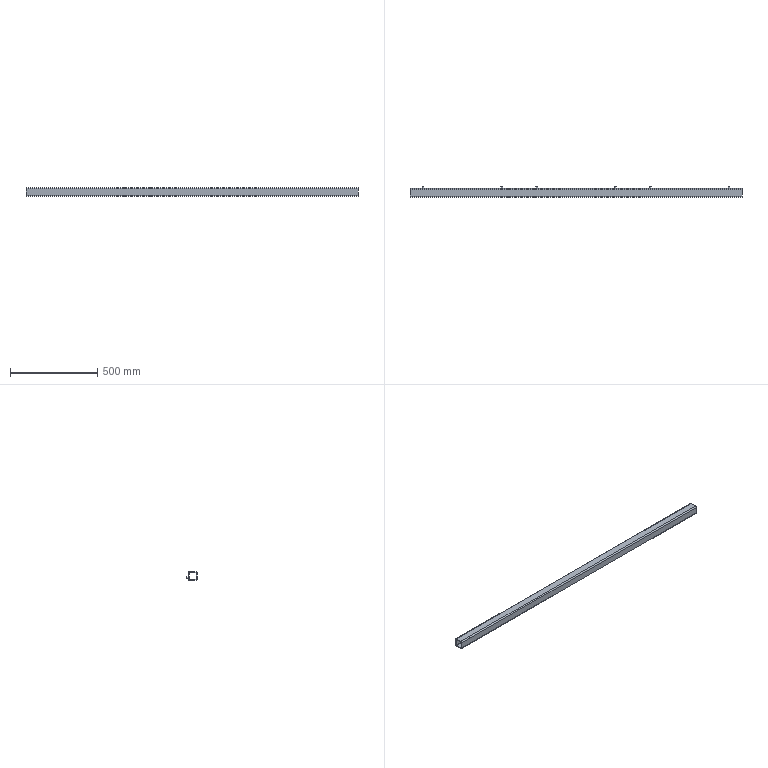Part | NX | 1 solid | 30 faces | box 1900 x 60 x 50 mm | volume 1641319 mm3 | plane 16 | cylinder 14 | commonest cylinder face diameters 10 x6 4 x4 14 x4
STEP:
#1=CARTESIAN_POINT('',(-425.,25.,-590.));
#2=VERTEX_POINT('',#1);
#3=CARTESIAN_POINT('',(-425.,25.,-585.));
#4=DIRECTION('',(0.,-1.,0.));
#5=DIRECTION('',(0.,0.,-1.));
#6=AXIS2_PLACEMENT_3D('',#3,#4,#5);
#7=CIRCLE('',#6,5.);
#8=EDGE_CURVE('',#2,#2,#7,.F.);
#9=ORIENTED_EDGE('',*,*,#8,.F.);
#10=EDGE_LOOP('',(#9));
#11=FACE_BOUND('',#10,.T.);
#12=CARTESIAN_POINT('',(225.,25.,-590.));
#13=VERTEX_POINT('',#12);
#14=CARTESIAN_POINT('',(225.,25.,-585.));
#15=DIRECTION('',(0.,-1.,0.));
#16=DIRECTION('',(0.,0.,-1.));
#17=AXIS2_PLACEMENT_3D('',#14,#15,#16);
#18=CIRCLE('',#17,5.);
#19=EDGE_CURVE('',#13,#13,#18,.F.);
#20=ORIENTED_EDGE('',*,*,#19,.F.);
#21=EDGE_LOOP('',(#20));
#22=FACE_BOUND('',#21,.T.);
#23=CARTESIAN_POINT('',(875.,25.,-590.));
#24=VERTEX_POINT('',#23);
#25=CARTESIAN_POINT('',(875.,25.,-585.));
#26=DIRECTION('',(0.,-1.,0.));
#27=DIRECTION('',(0.,0.,-1.));
#28=AXIS2_PLACEMENT_3D('',#25,#26,#27);
#29=CIRCLE('',#28,5.);
#30=EDGE_CURVE('',#24,#24,#29,.F.);
#31=ORIENTED_EDGE('',*,*,#30,.F.);
#32=EDGE_LOOP('',(#31));
#33=FACE_BOUND('',#32,.T.);
#34=CARTESIAN_POINT('',(950.,25.,-593.));
#35=VERTEX_POINT('',#34);
#36=CARTESIAN_POINT('',(950.,25.,-557.));
#37=VERTEX_POINT('',#36);
#38=CARTESIAN_POINT('',(950.,25.,-557.));
#39=DIRECTION('',(0.,0.,1.));
#40=VECTOR('',#39,1000.);
#41=LINE('',#38,#40);
#42=EDGE_CURVE('',#35,#37,#41,.T.);
#43=ORIENTED_EDGE('',*,*,#42,.F.);
#44=CARTESIAN_POINT('',(-950.,25.,-593.));
#45=VERTEX_POINT('',#44);
#46=CARTESIAN_POINT('',(-975.,25.,-593.));
#47=DIRECTION('',(1.,0.,0.));
#48=VECTOR('',#47,1000.);
#49=LINE('',#46,#48);
#50=EDGE_CURVE('',#45,#35,#49,.T.);
#51=ORIENTED_EDGE('',*,*,#50,.F.);
#52=CARTESIAN_POINT('',(-950.,25.,-557.));
#53=VERTEX_POINT('',#52);
#54=CARTESIAN_POINT('',(-950.,25.,-557.));
#55=DIRECTION('',(0.,0.,-1.));
#56=VECTOR('',#55,1000.);
#57=LINE('',#54,#56);
#58=EDGE_CURVE('',#53,#45,#57,.T.);
#59=ORIENTED_EDGE('',*,*,#58,.F.);
#60=CARTESIAN_POINT('',(-975.,25.,-557.));
#61=DIRECTION('',(1.,0.,0.));
#62=VECTOR('',#61,1000.);
#63=LINE('',#60,#62);
#64=EDGE_CURVE('',#53,#37,#63,.T.);
#65=ORIENTED_EDGE('',*,*,#64,.T.);
#66=EDGE_LOOP('',(#43,#51,#59,#65));
#67=FACE_BOUND('',#66,.T.);
#68=CARTESIAN_POINT('',(425.,25.,-590.));
#69=VERTEX_POINT('',#68);
#70=CARTESIAN_POINT('',(425.,25.,-585.));
#71=DIRECTION('',(0.,-1.,0.));
#72=DIRECTION('',(0.,0.,-1.));
#73=AXIS2_PLACEMENT_3D('',#70,#71,#72);
#74=CIRCLE('',#73,5.);
#75=EDGE_CURVE('',#69,#69,#74,.F.);
#76=ORIENTED_EDGE('',*,*,#75,.F.);
#77=EDGE_LOOP('',(#76));
#78=FACE_BOUND('',#77,.T.);
#79=CARTESIAN_POINT('',(-225.,25.,-590.));
#80=VERTEX_POINT('',#79);
#81=CARTESIAN_POINT('',(-225.,25.,-585.));
#82=DIRECTION('',(0.,-1.,0.));
#83=DIRECTION('',(0.,0.,-1.));
#84=AXIS2_PLACEMENT_3D('',#81,#82,#83);
#85=CIRCLE('',#84,5.);
#86=EDGE_CURVE('',#80,#80,#85,.F.);
#87=ORIENTED_EDGE('',*,*,#86,.F.);
#88=EDGE_LOOP('',(#87));
#89=FACE_BOUND('',#88,.T.);
#90=CARTESIAN_POINT('',(-875.,25.,-590.));
#91=VERTEX_POINT('',#90);
#92=CARTESIAN_POINT('',(-875.,25.,-585.));
#93=DIRECTION('',(0.,-1.,0.));
#94=DIRECTION('',(0.,0.,-1.));
#95=AXIS2_PLACEMENT_3D('',#92,#93,#94);
#96=CIRCLE('',#95,5.);
#97=EDGE_CURVE('',#91,#91,#96,.F.);
#98=ORIENTED_EDGE('',*,*,#97,.F.);
#99=EDGE_LOOP('',(#98));
#100=FACE_BOUND('',#99,.T.);
#101=CARTESIAN_POINT('',(-975.,25.,-557.));
#102=DIRECTION('',(0.,-1.,0.));
#103=DIRECTION('',(0.,0.,-1.));
#104=AXIS2_PLACEMENT_3D('',#101,#102,#103);
#105=PLANE('',#104);
#106=ADVANCED_FACE('',(#11,#22,#33,#67,#78,#89,#100),#105,.F.);
#107=CARTESIAN_POINT('',(-950.,-18.,-595.));
#108=VERTEX_POINT('',#107);
#109=CARTESIAN_POINT('',(950.,-18.,-595.));
#110=VERTEX_POINT('',#109);
#111=CARTESIAN_POINT('',(-975.,-18.,-595.));
#112=DIRECTION('',(1.,0.,0.));
#113=VECTOR('',#112,1000.);
#114=LINE('',#111,#113);
#115=EDGE_CURVE('',#108,#110,#114,.T.);
#116=ORIENTED_EDGE('',*,*,#115,.T.);
#117=CARTESIAN_POINT('',(950.,18.,-595.));
#118=VERTEX_POINT('',#117);
#119=CARTESIAN_POINT('',(950.,-18.,-595.));
#120=DIRECTION('',(0.,1.,0.));
#121=VECTOR('',#120,1000.);
#122=LINE('',#119,#121);
#123=EDGE_CURVE('',#110,#118,#122,.T.);
#124=ORIENTED_EDGE('',*,*,#123,.T.);
#125=CARTESIAN_POINT('',(-950.,18.,-595.));
#126=VERTEX_POINT('',#125);
#127=CARTESIAN_POINT('',(-975.,18.,-595.));
#128=DIRECTION('',(1.,0.,0.));
#129=VECTOR('',#128,1000.);
#130=LINE('',#127,#129);
#131=EDGE_CURVE('',#126,#118,#130,.T.);
#132=ORIENTED_EDGE('',*,*,#131,.F.);
#133=CARTESIAN_POINT('',(-950.,-18.,-595.));
#134=DIRECTION('',(0.,-1.,0.));
#135=VECTOR('',#134,1000.);
#136=LINE('',#133,#135);
#137=EDGE_CURVE('',#126,#108,#136,.T.);
#138=ORIENTED_EDGE('',*,*,#137,.T.);
#139=EDGE_LOOP('',(#116,#124,#132,#138));
#140=FACE_BOUND('',#139,.T.);
#141=CARTESIAN_POINT('',(-975.,-18.,-595.));
#142=DIRECTION('',(0.,0.,1.));
#143=DIRECTION('',(0.,-1.,0.));
#144=AXIS2_PLACEMENT_3D('',#141,#142,#143);
#145=PLANE('',#144);
#146=ADVANCED_FACE('',(#140),#145,.T.);
#147=CARTESIAN_POINT('',(-950.,-20.,-593.));
#148=VERTEX_POINT('',#147);
#149=CARTESIAN_POINT('',(950.,-20.,-593.));
#150=VERTEX_POINT('',#149);
#151=CARTESIAN_POINT('',(-975.,-20.,-593.));
#152=DIRECTION('',(1.,0.,0.));
#153=VECTOR('',#152,1000.);
#154=LINE('',#151,#153);
#155=EDGE_CURVE('',#148,#150,#154,.T.);
#156=ORIENTED_EDGE('',*,*,#155,.T.);
#157=CARTESIAN_POINT('',(950.,-18.,-593.));
#158=DIRECTION('',(1.,0.,0.));
#159=DIRECTION('',(0.,1.,0.));
#160=AXIS2_PLACEMENT_3D('',#157,#158,#159);
#161=CIRCLE('',#160,2.);
#162=EDGE_CURVE('',#150,#110,#161,.T.);
#163=ORIENTED_EDGE('',*,*,#162,.T.);
#164=ORIENTED_EDGE('',*,*,#115,.F.);
#165=CARTESIAN_POINT('',(-950.,-18.,-593.));
#166=DIRECTION('',(-1.,0.,0.));
#167=DIRECTION('',(0.,-1.,0.));
#168=AXIS2_PLACEMENT_3D('',#165,#166,#167);
#169=CIRCLE('',#168,2.);
#170=EDGE_CURVE('',#108,#148,#169,.T.);
#171=ORIENTED_EDGE('',*,*,#170,.T.);
#172=EDGE_LOOP('',(#156,#163,#164,#171));
#173=FACE_BOUND('',#172,.T.);
#174=CARTESIAN_POINT('',(-975.,-18.,-593.));
#175=DIRECTION('',(1.,0.,0.));
#176=DIRECTION('',(0.,0.,-1.));
#177=AXIS2_PLACEMENT_3D('',#174,#175,#176);
#178=CYLINDRICAL_SURFACE('',#177,2.);
#179=ADVANCED_FACE('',(#173),#178,.F.);
#180=CARTESIAN_POINT('',(-950.,-20.,-557.));
#181=VERTEX_POINT('',#180);
#182=CARTESIAN_POINT('',(950.,-20.,-557.));
#183=VERTEX_POINT('',#182);
#184=CARTESIAN_POINT('',(-975.,-20.,-557.));
#185=DIRECTION('',(1.,0.,0.));
#186=VECTOR('',#185,1000.);
#187=LINE('',#184,#186);
#188=EDGE_CURVE('',#181,#183,#187,.T.);
#189=ORIENTED_EDGE('',*,*,#188,.T.);
#190=CARTESIAN_POINT('',(950.,-20.,-593.));
#191=DIRECTION('',(0.,0.,-1.));
#192=VECTOR('',#191,1000.);
#193=LINE('',#190,#192);
#194=EDGE_CURVE('',#183,#150,#193,.T.);
#195=ORIENTED_EDGE('',*,*,#194,.T.);
#196=ORIENTED_EDGE('',*,*,#155,.F.);
#197=CARTESIAN_POINT('',(-950.,-20.,-593.));
#198=DIRECTION('',(0.,0.,1.));
#199=VECTOR('',#198,1000.);
#200=LINE('',#197,#199);
#201=EDGE_CURVE('',#148,#181,#200,.T.);
#202=ORIENTED_EDGE('',*,*,#201,.T.);
#203=EDGE_LOOP('',(#189,#195,#196,#202));
#204=FACE_BOUND('',#203,.T.);
#205=CARTESIAN_POINT('',(-975.,-20.,-593.));
#206=DIRECTION('',(0.,1.,0.));
#207=DIRECTION('',(0.,0.,1.));
#208=AXIS2_PLACEMENT_3D('',#205,#206,#207);
#209=PLANE('',#208);
#210=ADVANCED_FACE('',(#204),#209,.T.);
#211=CARTESIAN_POINT('',(-950.,-18.,-555.));
#212=VERTEX_POINT('',#211);
#213=CARTESIAN_POINT('',(950.,-18.,-555.));
#214=VERTEX_POINT('',#213);
#215=CARTESIAN_POINT('',(-975.,-18.,-555.));
#216=DIRECTION('',(1.,0.,0.));
#217=VECTOR('',#216,1000.);
#218=LINE('',#215,#217);
#219=EDGE_CURVE('',#212,#214,#218,.T.);
#220=ORIENTED_EDGE('',*,*,#219,.T.);
#221=CARTESIAN_POINT('',(950.,-18.,-557.));
#222=DIRECTION('',(1.,0.,0.));
#223=DIRECTION('',(0.,1.,0.));
#224=AXIS2_PLACEMENT_3D('',#221,#222,#223);
#225=CIRCLE('',#224,2.);
#226=EDGE_CURVE('',#214,#183,#225,.T.);
#227=ORIENTED_EDGE('',*,*,#226,.T.);
#228=ORIENTED_EDGE('',*,*,#188,.F.);
#229=CARTESIAN_POINT('',(-950.,-18.,-557.));
#230=DIRECTION('',(-1.,0.,0.));
#231=DIRECTION('',(0.,-1.,0.));
#232=AXIS2_PLACEMENT_3D('',#229,#230,#231);
#233=CIRCLE('',#232,2.);
#234=EDGE_CURVE('',#181,#212,#233,.T.);
#235=ORIENTED_EDGE('',*,*,#234,.T.);
#236=EDGE_LOOP('',(#220,#227,#228,#235));
#237=FACE_BOUND('',#236,.T.);
#238=CARTESIAN_POINT('',(-975.,-18.,-557.));
#239=DIRECTION('',(1.,0.,0.));
#240=DIRECTION('',(0.,0.,-1.));
#241=AXIS2_PLACEMENT_3D('',#238,#239,#240);
#242=CYLINDRICAL_SURFACE('',#241,2.);
#243=ADVANCED_FACE('',(#237),#242,.F.);
#244=CARTESIAN_POINT('',(-950.,18.,-555.));
#245=VERTEX_POINT('',#244);
#246=CARTESIAN_POINT('',(950.,18.,-555.));
#247=VERTEX_POINT('',#246);
#248=CARTESIAN_POINT('',(-975.,18.,-555.));
#249=DIRECTION('',(1.,0.,0.));
#250=VECTOR('',#249,1000.);
#251=LINE('',#248,#250);
#252=EDGE_CURVE('',#245,#247,#251,.T.);
#253=ORIENTED_EDGE('',*,*,#252,.T.);
#254=CARTESIAN_POINT('',(950.,18.,-555.));
#255=DIRECTION('',(0.,-1.,0.));
#256=VECTOR('',#255,1000.);
#257=LINE('',#254,#256);
#258=EDGE_CURVE('',#247,#214,#257,.T.);
#259=ORIENTED_EDGE('',*,*,#258,.T.);
#260=ORIENTED_EDGE('',*,*,#219,.F.);
#261=CARTESIAN_POINT('',(-950.,18.,-555.));
#262=DIRECTION('',(0.,1.,0.));
#263=VECTOR('',#262,1000.);
#264=LINE('',#261,#263);
#265=EDGE_CURVE('',#212,#245,#264,.T.);
#266=ORIENTED_EDGE('',*,*,#265,.T.);
#267=EDGE_LOOP('',(#253,#259,#260,#266));
#268=FACE_BOUND('',#267,.T.);
#269=CARTESIAN_POINT('',(-975.,18.,-555.));
#270=DIRECTION('',(0.,0.,-1.));
#271=DIRECTION('',(0.,1.,0.));
#272=AXIS2_PLACEMENT_3D('',#269,#270,#271);
#273=PLANE('',#272);
#274=ADVANCED_FACE('',(#268),#273,.T.);
#275=CARTESIAN_POINT('',(-950.,20.,-557.));
#276=VERTEX_POINT('',#275);
#277=CARTESIAN_POINT('',(950.,20.,-557.));
#278=VERTEX_POINT('',#277);
#279=CARTESIAN_POINT('',(-975.,20.,-557.));
#280=DIRECTION('',(1.,0.,0.));
#281=VECTOR('',#280,1000.);
#282=LINE('',#279,#281);
#283=EDGE_CURVE('',#276,#278,#282,.T.);
#284=ORIENTED_EDGE('',*,*,#283,.T.);
#285=CARTESIAN_POINT('',(950.,18.,-557.));
#286=DIRECTION('',(1.,0.,0.));
#287=DIRECTION('',(0.,1.,0.));
#288=AXIS2_PLACEMENT_3D('',#285,#286,#287);
#289=CIRCLE('',#288,2.);
#290=EDGE_CURVE('',#278,#247,#289,.T.);
#291=ORIENTED_EDGE('',*,*,#290,.T.);
#292=ORIENTED_EDGE('',*,*,#252,.F.);
#293=CARTESIAN_POINT('',(-950.,18.,-557.));
#294=DIRECTION('',(-1.,0.,0.));
#295=DIRECTION('',(0.,-1.,0.));
#296=AXIS2_PLACEMENT_3D('',#293,#294,#295);
#297=CIRCLE('',#296,2.);
#298=EDGE_CURVE('',#245,#276,#297,.T.);
#299=ORIENTED_EDGE('',*,*,#298,.T.);
#300=EDGE_LOOP('',(#284,#291,#292,#299));
#301=FACE_BOUND('',#300,.T.);
#302=CARTESIAN_POINT('',(-975.,18.,-557.));
#303=DIRECTION('',(1.,0.,0.));
#304=DIRECTION('',(0.,0.,-1.));
#305=AXIS2_PLACEMENT_3D('',#302,#303,#304);
#306=CYLINDRICAL_SURFACE('',#305,2.);
#307=ADVANCED_FACE('',(#301),#306,.F.);
#308=CARTESIAN_POINT('',(-950.,20.,-593.));
#309=VERTEX_POINT('',#308);
#310=CARTESIAN_POINT('',(950.,20.,-593.));
#311=VERTEX_POINT('',#310);
#312=CARTESIAN_POINT('',(-975.,20.,-593.));
#313=DIRECTION('',(1.,0.,0.));
#314=VECTOR('',#313,1000.);
#315=LINE('',#312,#314);
#316=EDGE_CURVE('',#309,#311,#315,.T.);
#317=ORIENTED_EDGE('',*,*,#316,.T.);
#318=CARTESIAN_POINT('',(950.,20.,-557.));
#319=DIRECTION('',(0.,0.,1.));
#320=VECTOR('',#319,1000.);
#321=LINE('',#318,#320);
#322=EDGE_CURVE('',#311,#278,#321,.T.);
#323=ORIENTED_EDGE('',*,*,#322,.T.);
#324=ORIENTED_EDGE('',*,*,#283,.F.);
#325=CARTESIAN_POINT('',(-950.,20.,-557.));
#326=DIRECTION('',(0.,0.,-1.));
#327=VECTOR('',#326,1000.);
#328=LINE('',#325,#327);
#329=EDGE_CURVE('',#276,#309,#328,.T.);
#330=ORIENTED_EDGE('',*,*,#329,.T.);
#331=EDGE_LOOP('',(#317,#323,#324,#330));
#332=FACE_BOUND('',#331,.T.);
#333=CARTESIAN_POINT('',(-975.,20.,-557.));
#334=DIRECTION('',(0.,-1.,0.));
#335=DIRECTION('',(0.,0.,-1.));
#336=AXIS2_PLACEMENT_3D('',#333,#334,#335);
#337=PLANE('',#336);
#338=ADVANCED_FACE('',(#332),#337,.T.);
#339=ORIENTED_EDGE('',*,*,#131,.T.);
#340=CARTESIAN_POINT('',(950.,18.,-593.));
#341=DIRECTION('',(1.,0.,0.));
#342=DIRECTION('',(0.,1.,0.));
#343=AXIS2_PLACEMENT_3D('',#340,#341,#342);
#344=CIRCLE('',#343,2.);
#345=EDGE_CURVE('',#118,#311,#344,.T.);
#346=ORIENTED_EDGE('',*,*,#345,.T.);
#347=ORIENTED_EDGE('',*,*,#316,.F.);
#348=CARTESIAN_POINT('',(-950.,18.,-593.));
#349=DIRECTION('',(-1.,0.,0.));
#350=DIRECTION('',(0.,-1.,0.));
#351=AXIS2_PLACEMENT_3D('',#348,#349,#350);
#352=CIRCLE('',#351,2.);
#353=EDGE_CURVE('',#309,#126,#352,.T.);
#354=ORIENTED_EDGE('',*,*,#353,.T.);
#355=EDGE_LOOP('',(#339,#346,#347,#354));
#356=FACE_BOUND('',#355,.T.);
#357=CARTESIAN_POINT('',(-975.,18.,-593.));
#358=DIRECTION('',(1.,0.,0.));
#359=DIRECTION('',(0.,0.,-1.));
#360=AXIS2_PLACEMENT_3D('',#357,#358,#359);
#361=CYLINDRICAL_SURFACE('',#360,2.);
#362=ADVANCED_FACE('',(#356),#361,.F.);
#363=ORIENTED_EDGE('',*,*,#329,.F.);
#364=ORIENTED_EDGE('',*,*,#298,.F.);
#365=ORIENTED_EDGE('',*,*,#265,.F.);
#366=ORIENTED_EDGE('',*,*,#234,.F.);
#367=ORIENTED_EDGE('',*,*,#201,.F.);
#368=ORIENTED_EDGE('',*,*,#170,.F.);
#369=ORIENTED_EDGE('',*,*,#137,.F.);
#370=ORIENTED_EDGE('',*,*,#353,.F.);
#371=EDGE_LOOP('',(#363,#364,#365,#366,#367,#368,#369,#370));
#372=FACE_BOUND('',#371,.T.);
#373=CARTESIAN_POINT('',(-950.,18.,-550.));
#374=VERTEX_POINT('',#373);
#375=CARTESIAN_POINT('',(-950.,18.,-557.));
#376=DIRECTION('',(-1.,0.,0.));
#377=DIRECTION('',(0.,-1.,0.));
#378=AXIS2_PLACEMENT_3D('',#375,#376,#377);
#379=CIRCLE('',#378,7.);
#380=EDGE_CURVE('',#374,#53,#379,.T.);
#381=ORIENTED_EDGE('',*,*,#380,.T.);
#382=ORIENTED_EDGE('',*,*,#58,.T.);
#383=CARTESIAN_POINT('',(-950.,18.,-600.));
#384=VERTEX_POINT('',#383);
#385=CARTESIAN_POINT('',(-950.,18.,-593.));
#386=DIRECTION('',(-1.,0.,0.));
#387=DIRECTION('',(0.,-1.,0.));
#388=AXIS2_PLACEMENT_3D('',#385,#386,#387);
#389=CIRCLE('',#388,7.);
#390=EDGE_CURVE('',#45,#384,#389,.T.);
#391=ORIENTED_EDGE('',*,*,#390,.T.);
#392=CARTESIAN_POINT('',(-950.,-18.,-600.));
#393=VERTEX_POINT('',#392);
#394=CARTESIAN_POINT('',(-950.,0.,-600.));
#395=DIRECTION('',(0.,1.,0.));
#396=VECTOR('',#395,1000.);
#397=LINE('',#394,#396);
#398=EDGE_CURVE('',#393,#384,#397,.T.);
#399=ORIENTED_EDGE('',*,*,#398,.F.);
#400=CARTESIAN_POINT('',(-950.,-25.,-593.));
#401=VERTEX_POINT('',#400);
#402=CARTESIAN_POINT('',(-950.,-18.,-593.));
#403=DIRECTION('',(-1.,0.,0.));
#404=DIRECTION('',(0.,-1.,0.));
#405=AXIS2_PLACEMENT_3D('',#402,#403,#404);
#406=CIRCLE('',#405,7.);
#407=EDGE_CURVE('',#393,#401,#406,.T.);
#408=ORIENTED_EDGE('',*,*,#407,.T.);
#409=CARTESIAN_POINT('',(-950.,-25.,-557.));
#410=VERTEX_POINT('',#409);
#411=CARTESIAN_POINT('',(-950.,-25.,-593.));
#412=DIRECTION('',(0.,0.,1.));
#413=VECTOR('',#412,1000.);
#414=LINE('',#411,#413);
#415=EDGE_CURVE('',#401,#410,#414,.T.);
#416=ORIENTED_EDGE('',*,*,#415,.T.);
#417=CARTESIAN_POINT('',(-950.,-18.,-550.));
#418=VERTEX_POINT('',#417);
#419=CARTESIAN_POINT('',(-950.,-18.,-557.));
#420=DIRECTION('',(-1.,0.,0.));
#421=DIRECTION('',(0.,-1.,0.));
#422=AXIS2_PLACEMENT_3D('',#419,#420,#421);
#423=CIRCLE('',#422,7.);
#424=EDGE_CURVE('',#410,#418,#423,.T.);
#425=ORIENTED_EDGE('',*,*,#424,.T.);
#426=CARTESIAN_POINT('',(-950.,18.,-550.));
#427=DIRECTION('',(0.,1.,0.));
#428=VECTOR('',#427,1000.);
#429=LINE('',#426,#428);
#430=EDGE_CURVE('',#418,#374,#429,.T.);
#431=ORIENTED_EDGE('',*,*,#430,.T.);
#432=EDGE_LOOP('',(#381,#382,#391,#399,#408,#416,#425,#431));
#433=FACE_BOUND('',#432,.T.);
#434=CARTESIAN_POINT('',(-950.,0.,-557.));
#435=DIRECTION('',(-1.,0.,0.));
#436=DIRECTION('',(0.,-1.,0.));
#437=AXIS2_PLACEMENT_3D('',#434,#435,#436);
#438=PLANE('',#437);
#439=ADVANCED_FACE('',(#372,#433),#438,.T.);
#440=CARTESIAN_POINT('',(950.,18.,-550.));
#441=VERTEX_POINT('',#440);
#442=CARTESIAN_POINT('',(950.,-18.,-550.));
#443=VERTEX_POINT('',#442);
#444=CARTESIAN_POINT('',(950.,18.,-550.));
#445=DIRECTION('',(0.,-1.,0.));
#446=VECTOR('',#445,1000.);
#447=LINE('',#444,#446);
#448=EDGE_CURVE('',#441,#443,#447,.T.);
#449=ORIENTED_EDGE('',*,*,#448,.F.);
#450=CARTESIAN_POINT('',(-975.,18.,-550.));
#451=DIRECTION('',(1.,0.,0.));
#452=VECTOR('',#451,1000.);
#453=LINE('',#450,#452);
#454=EDGE_CURVE('',#374,#441,#453,.T.);
#455=ORIENTED_EDGE('',*,*,#454,.F.);
#456=ORIENTED_EDGE('',*,*,#430,.F.);
#457=CARTESIAN_POINT('',(-975.,-18.,-550.));
#458=DIRECTION('',(1.,0.,0.));
#459=VECTOR('',#458,1000.);
#460=LINE('',#457,#459);
#461=EDGE_CURVE('',#418,#443,#460,.T.);
#462=ORIENTED_EDGE('',*,*,#461,.T.);
#463=EDGE_LOOP('',(#449,#455,#456,#462));
#464=FACE_BOUND('',#463,.T.);
#465=CARTESIAN_POINT('',(-975.,18.,-550.));
#466=DIRECTION('',(0.,0.,-1.));
#467=DIRECTION('',(0.,1.,0.));
#468=AXIS2_PLACEMENT_3D('',#465,#466,#467);
#469=PLANE('',#468);
#470=ADVANCED_FACE('',(#464),#469,.F.);
#471=CARTESIAN_POINT('',(950.,-25.,-557.));
#472=VERTEX_POINT('',#471);
#473=CARTESIAN_POINT('',(950.,-18.,-557.));
#474=DIRECTION('',(1.,0.,0.));
#475=DIRECTION('',(0.,1.,0.));
#476=AXIS2_PLACEMENT_3D('',#473,#474,#475);
#477=CIRCLE('',#476,7.);
#478=EDGE_CURVE('',#443,#472,#477,.T.);
#479=ORIENTED_EDGE('',*,*,#478,.F.);
#480=ORIENTED_EDGE('',*,*,#461,.F.);
#481=ORIENTED_EDGE('',*,*,#424,.F.);
#482=CARTESIAN_POINT('',(-975.,-25.,-557.));
#483=DIRECTION('',(1.,0.,0.));
#484=VECTOR('',#483,1000.);
#485=LINE('',#482,#484);
#486=EDGE_CURVE('',#410,#472,#485,.T.);
#487=ORIENTED_EDGE('',*,*,#486,.T.);
#488=EDGE_LOOP('',(#479,#480,#481,#487));
#489=FACE_BOUND('',#488,.T.);
#490=CARTESIAN_POINT('',(-975.,-18.,-557.));
#491=DIRECTION('',(1.,0.,0.));
#492=DIRECTION('',(0.,0.,-1.));
#493=AXIS2_PLACEMENT_3D('',#490,#491,#492);
#494=CYLINDRICAL_SURFACE('',#493,7.);
#495=ADVANCED_FACE('',(#489),#494,.T.);
#496=CARTESIAN_POINT('',(950.,-25.,-593.));
#497=VERTEX_POINT('',#496);
#498=CARTESIAN_POINT('',(950.,-25.,-593.));
#499=DIRECTION('',(0.,0.,-1.));
#500=VECTOR('',#499,1000.);
#501=LINE('',#498,#500);
#502=EDGE_CURVE('',#472,#497,#501,.T.);
#503=ORIENTED_EDGE('',*,*,#502,.F.);
#504=ORIENTED_EDGE('',*,*,#486,.F.);
#505=ORIENTED_EDGE('',*,*,#415,.F.);
#506=CARTESIAN_POINT('',(-975.,-25.,-593.));
#507=DIRECTION('',(1.,0.,0.));
#508=VECTOR('',#507,1000.);
#509=LINE('',#506,#508);
#510=EDGE_CURVE('',#401,#497,#509,.T.);
#511=ORIENTED_EDGE('',*,*,#510,.T.);
#512=EDGE_LOOP('',(#503,#504,#505,#511));
#513=FACE_BOUND('',#512,.T.);
#514=CARTESIAN_POINT('',(-975.,-25.,-593.));
#515=DIRECTION('',(0.,1.,0.));
#516=DIRECTION('',(0.,0.,1.));
#517=AXIS2_PLACEMENT_3D('',#514,#515,#516);
#518=PLANE('',#517);
#519=ADVANCED_FACE('',(#513),#518,.F.);
#520=CARTESIAN_POINT('',(950.,-18.,-600.));
#521=VERTEX_POINT('',#520);
#522=CARTESIAN_POINT('',(950.,-18.,-593.));
#523=DIRECTION('',(1.,0.,0.));
#524=DIRECTION('',(0.,1.,0.));
#525=AXIS2_PLACEMENT_3D('',#522,#523,#524);
#526=CIRCLE('',#525,7.);
#527=EDGE_CURVE('',#497,#521,#526,.T.);
#528=ORIENTED_EDGE('',*,*,#527,.F.);
#529=ORIENTED_EDGE('',*,*,#510,.F.);
#530=ORIENTED_EDGE('',*,*,#407,.F.);
#531=CARTESIAN_POINT('',(-975.,-18.,-600.));
#532=DIRECTION('',(1.,0.,0.));
#533=VECTOR('',#532,1000.);
#534=LINE('',#531,#533);
#535=EDGE_CURVE('',#393,#521,#534,.T.);
#536=ORIENTED_EDGE('',*,*,#535,.T.);
#537=EDGE_LOOP('',(#528,#529,#530,#536));
#538=FACE_BOUND('',#537,.T.);
#539=CARTESIAN_POINT('',(-975.,-18.,-593.));
#540=DIRECTION('',(1.,0.,0.));
#541=DIRECTION('',(0.,0.,-1.));
#542=AXIS2_PLACEMENT_3D('',#539,#540,#541);
#543=CYLINDRICAL_SURFACE('',#542,7.);
#544=ADVANCED_FACE('',(#538),#543,.T.);
#545=CARTESIAN_POINT('',(950.,18.,-600.));
#546=VERTEX_POINT('',#545);
#547=CARTESIAN_POINT('',(950.,0.,-600.));
#548=DIRECTION('',(0.,1.,0.));
#549=VECTOR('',#548,1000.);
#550=LINE('',#547,#549);
#551=EDGE_CURVE('',#521,#546,#550,.T.);
#552=ORIENTED_EDGE('',*,*,#551,.F.);
#553=ORIENTED_EDGE('',*,*,#535,.F.);
#554=ORIENTED_EDGE('',*,*,#398,.T.);
#555=CARTESIAN_POINT('',(-975.,18.,-600.));
#556=DIRECTION('',(1.,0.,0.));
#557=VECTOR('',#556,1000.);
#558=LINE('',#555,#557);
#559=EDGE_CURVE('',#384,#546,#558,.T.);
#560=ORIENTED_EDGE('',*,*,#559,.T.);
#561=EDGE_LOOP('',(#552,#553,#554,#560));
#562=FACE_BOUND('',#561,.T.);
#563=CARTESIAN_POINT('',(-975.,-18.,-600.));
#564=DIRECTION('',(0.,0.,1.));
#565=DIRECTION('',(0.,-1.,0.));
#566=AXIS2_PLACEMENT_3D('',#563,#564,#565);
#567=PLANE('',#566);
#568=ADVANCED_FACE('',(#562),#567,.F.);
#569=CARTESIAN_POINT('',(950.,18.,-593.));
#570=DIRECTION('',(1.,0.,0.));
#571=DIRECTION('',(0.,1.,0.));
#572=AXIS2_PLACEMENT_3D('',#569,#570,#571);
#573=CIRCLE('',#572,7.);
#574=EDGE_CURVE('',#546,#35,#573,.T.);
#575=ORIENTED_EDGE('',*,*,#574,.F.);
#576=ORIENTED_EDGE('',*,*,#559,.F.);
#577=ORIENTED_EDGE('',*,*,#390,.F.);
#578=ORIENTED_EDGE('',*,*,#50,.T.);
#579=EDGE_LOOP('',(#575,#576,#577,#578));
#580=FACE_BOUND('',#579,.T.);
#581=CARTESIAN_POINT('',(-975.,18.,-593.));
#582=DIRECTION('',(1.,0.,0.));
#583=DIRECTION('',(0.,0.,-1.));
#584=AXIS2_PLACEMENT_3D('',#581,#582,#583);
#585=CYLINDRICAL_SURFACE('',#584,7.);
#586=ADVANCED_FACE('',(#580),#585,.T.);
#587=CARTESIAN_POINT('',(950.,18.,-557.));
#588=DIRECTION('',(1.,0.,0.));
#589=DIRECTION('',(0.,1.,0.));
#590=AXIS2_PLACEMENT_3D('',#587,#588,#589);
#591=CIRCLE('',#590,7.);
#592=EDGE_CURVE('',#37,#441,#591,.T.);
#593=ORIENTED_EDGE('',*,*,#592,.F.);
#594=ORIENTED_EDGE('',*,*,#64,.F.);
#595=ORIENTED_EDGE('',*,*,#380,.F.);
#596=ORIENTED_EDGE('',*,*,#454,.T.);
#597=EDGE_LOOP('',(#593,#594,#595,#596));
#598=FACE_BOUND('',#597,.T.);
#599=CARTESIAN_POINT('',(-975.,18.,-557.));
#600=DIRECTION('',(1.,0.,0.));
#601=DIRECTION('',(0.,0.,-1.));
#602=AXIS2_PLACEMENT_3D('',#599,#600,#601);
#603=CYLINDRICAL_SURFACE('',#602,7.);
#604=ADVANCED_FACE('',(#598),#603,.T.);
#605=ORIENTED_EDGE('',*,*,#123,.F.);
#606=ORIENTED_EDGE('',*,*,#162,.F.);
#607=ORIENTED_EDGE('',*,*,#194,.F.);
#608=ORIENTED_EDGE('',*,*,#226,.F.);
#609=ORIENTED_EDGE('',*,*,#258,.F.);
#610=ORIENTED_EDGE('',*,*,#290,.F.);
#611=ORIENTED_EDGE('',*,*,#322,.F.);
#612=ORIENTED_EDGE('',*,*,#345,.F.);
#613=EDGE_LOOP('',(#605,#606,#607,#608,#609,#610,#611,#612));
#614=FACE_BOUND('',#613,.T.);
#615=ORIENTED_EDGE('',*,*,#592,.T.);
#616=ORIENTED_EDGE('',*,*,#448,.T.);
#617=ORIENTED_EDGE('',*,*,#478,.T.);
#618=ORIENTED_EDGE('',*,*,#502,.T.);
#619=ORIENTED_EDGE('',*,*,#527,.T.);
#620=ORIENTED_EDGE('',*,*,#551,.T.);
#621=ORIENTED_EDGE('',*,*,#574,.T.);
#622=ORIENTED_EDGE('',*,*,#42,.T.);
#623=EDGE_LOOP('',(#615,#616,#617,#618,#619,#620,#621,#622));
#624=FACE_BOUND('',#623,.T.);
#625=CARTESIAN_POINT('',(950.,0.,-593.));
#626=DIRECTION('',(1.,0.,0.));
#627=DIRECTION('',(0.,1.,0.));
#628=AXIS2_PLACEMENT_3D('',#625,#626,#627);
#629=PLANE('',#628);
#630=ADVANCED_FACE('',(#614,#624),#629,.T.);
#631=CARTESIAN_POINT('',(875.,35.,-580.));
#632=VERTEX_POINT('',#631);
#633=CARTESIAN_POINT('',(875.,35.,-585.));
#634=DIRECTION('',(0.,1.,0.));
#635=DIRECTION('',(0.,0.,1.));
#636=AXIS2_PLACEMENT_3D('',#633,#634,#635);
#637=CIRCLE('',#636,5.);
#638=EDGE_CURVE('',#632,#632,#637,.T.);
#639=ORIENTED_EDGE('',*,*,#638,.F.);
#640=EDGE_LOOP('',(#639));
#641=FACE_BOUND('',#640,.T.);
#642=ORIENTED_EDGE('',*,*,#30,.T.);
#643=EDGE_LOOP('',(#642));
#644=FACE_BOUND('',#643,.T.);
#645=CARTESIAN_POINT('',(875.,35.,-585.));
#646=DIRECTION('',(0.,-1.,0.));
#647=DIRECTION('',(0.,0.,-1.));
#648=AXIS2_PLACEMENT_3D('',#645,#646,#647);
#649=CYLINDRICAL_SURFACE('',#648,5.);
#650=ADVANCED_FACE('',(#641,#644),#649,.T.);
#651=ORIENTED_EDGE('',*,*,#638,.T.);
#652=EDGE_LOOP('',(#651));
#653=FACE_BOUND('',#652,.T.);
#654=CARTESIAN_POINT('',(875.,35.,-585.));
#655=DIRECTION('',(0.,1.,0.));
#656=DIRECTION('',(0.,0.,1.));
#657=AXIS2_PLACEMENT_3D('',#654,#655,#656);
#658=PLANE('',#657);
#659=ADVANCED_FACE('',(#653),#658,.T.);
#660=CARTESIAN_POINT('',(425.,35.,-580.));
#661=VERTEX_POINT('',#660);
#662=CARTESIAN_POINT('',(425.,35.,-585.));
#663=DIRECTION('',(0.,1.,0.));
#664=DIRECTION('',(0.,0.,1.));
#665=AXIS2_PLACEMENT_3D('',#662,#663,#664);
#666=CIRCLE('',#665,5.);
#667=EDGE_CURVE('',#661,#661,#666,.T.);
#668=ORIENTED_EDGE('',*,*,#667,.F.);
#669=EDGE_LOOP('',(#668));
#670=FACE_BOUND('',#669,.T.);
#671=ORIENTED_EDGE('',*,*,#75,.T.);
#672=EDGE_LOOP('',(#671));
#673=FACE_BOUND('',#672,.T.);
#674=CARTESIAN_POINT('',(425.,35.,-585.));
#675=DIRECTION('',(0.,-1.,0.));
#676=DIRECTION('',(0.,0.,-1.));
#677=AXIS2_PLACEMENT_3D('',#674,#675,#676);
#678=CYLINDRICAL_SURFACE('',#677,5.);
#679=ADVANCED_FACE('',(#670,#673),#678,.T.);
#680=ORIENTED_EDGE('',*,*,#667,.T.);
#681=EDGE_LOOP('',(#680));
#682=FACE_BOUND('',#681,.T.);
#683=CARTESIAN_POINT('',(425.,35.,-585.));
#684=DIRECTION('',(0.,1.,0.));
#685=DIRECTION('',(0.,0.,1.));
#686=AXIS2_PLACEMENT_3D('',#683,#684,#685);
#687=PLANE('',#686);
#688=ADVANCED_FACE('',(#682),#687,.T.);
#689=CARTESIAN_POINT('',(225.,35.,-580.));
#690=VERTEX_POINT('',#689);
#691=CARTESIAN_POINT('',(225.,35.,-585.));
#692=DIRECTION('',(0.,1.,0.));
#693=DIRECTION('',(0.,0.,1.));
#694=AXIS2_PLACEMENT_3D('',#691,#692,#693);
#695=CIRCLE('',#694,5.);
#696=EDGE_CURVE('',#690,#690,#695,.T.);
#697=ORIENTED_EDGE('',*,*,#696,.F.);
#698=EDGE_LOOP('',(#697));
#699=FACE_BOUND('',#698,.T.);
#700=ORIENTED_EDGE('',*,*,#19,.T.);
#701=EDGE_LOOP('',(#700));
#702=FACE_BOUND('',#701,.T.);
#703=CARTESIAN_POINT('',(225.,35.,-585.));
#704=DIRECTION('',(0.,-1.,0.));
#705=DIRECTION('',(0.,0.,-1.));
#706=AXIS2_PLACEMENT_3D('',#703,#704,#705);
#707=CYLINDRICAL_SURFACE('',#706,5.);
#708=ADVANCED_FACE('',(#699,#702),#707,.T.);
#709=ORIENTED_EDGE('',*,*,#696,.T.);
#710=EDGE_LOOP('',(#709));
#711=FACE_BOUND('',#710,.T.);
#712=CARTESIAN_POINT('',(225.,35.,-585.));
#713=DIRECTION('',(0.,1.,0.));
#714=DIRECTION('',(0.,0.,1.));
#715=AXIS2_PLACEMENT_3D('',#712,#713,#714);
#716=PLANE('',#715);
#717=ADVANCED_FACE('',(#711),#716,.T.);
#718=CARTESIAN_POINT('',(-225.,35.,-580.));
#719=VERTEX_POINT('',#718);
#720=CARTESIAN_POINT('',(-225.,35.,-585.));
#721=DIRECTION('',(0.,1.,0.));
#722=DIRECTION('',(0.,0.,1.));
#723=AXIS2_PLACEMENT_3D('',#720,#721,#722);
#724=CIRCLE('',#723,5.);
#725=EDGE_CURVE('',#719,#719,#724,.T.);
#726=ORIENTED_EDGE('',*,*,#725,.F.);
#727=EDGE_LOOP('',(#726));
#728=FACE_BOUND('',#727,.T.);
#729=ORIENTED_EDGE('',*,*,#86,.T.);
#730=EDGE_LOOP('',(#729));
#731=FACE_BOUND('',#730,.T.);
#732=CARTESIAN_POINT('',(-225.,35.,-585.));
#733=DIRECTION('',(0.,-1.,0.));
#734=DIRECTION('',(0.,0.,-1.));
#735=AXIS2_PLACEMENT_3D('',#732,#733,#734);
#736=CYLINDRICAL_SURFACE('',#735,5.);
#737=ADVANCED_FACE('',(#728,#731),#736,.T.);
#738=ORIENTED_EDGE('',*,*,#725,.T.);
#739=EDGE_LOOP('',(#738));
#740=FACE_BOUND('',#739,.T.);
#741=CARTESIAN_POINT('',(-225.,35.,-585.));
#742=DIRECTION('',(0.,1.,0.));
#743=DIRECTION('',(0.,0.,1.));
#744=AXIS2_PLACEMENT_3D('',#741,#742,#743);
#745=PLANE('',#744);
#746=ADVANCED_FACE('',(#740),#745,.T.);
#747=CARTESIAN_POINT('',(-425.,35.,-580.));
#748=VERTEX_POINT('',#747);
#749=CARTESIAN_POINT('',(-425.,35.,-585.));
#750=DIRECTION('',(0.,1.,0.));
#751=DIRECTION('',(0.,0.,1.));
#752=AXIS2_PLACEMENT_3D('',#749,#750,#751);
#753=CIRCLE('',#752,5.);
#754=EDGE_CURVE('',#748,#748,#753,.T.);
#755=ORIENTED_EDGE('',*,*,#754,.F.);
#756=EDGE_LOOP('',(#755));
#757=FACE_BOUND('',#756,.T.);
#758=ORIENTED_EDGE('',*,*,#8,.T.);
#759=EDGE_LOOP('',(#758));
#760=FACE_BOUND('',#759,.T.);
#761=CARTESIAN_POINT('',(-425.,35.,-585.));
#762=DIRECTION('',(0.,-1.,0.));
#763=DIRECTION('',(0.,0.,-1.));
#764=AXIS2_PLACEMENT_3D('',#761,#762,#763);
#765=CYLINDRICAL_SURFACE('',#764,5.);
#766=ADVANCED_FACE('',(#757,#760),#765,.T.);
#767=ORIENTED_EDGE('',*,*,#754,.T.);
#768=EDGE_LOOP('',(#767));
#769=FACE_BOUND('',#768,.T.);
#770=CARTESIAN_POINT('',(-425.,35.,-585.));
#771=DIRECTION('',(0.,1.,0.));
#772=DIRECTION('',(0.,0.,1.));
#773=AXIS2_PLACEMENT_3D('',#770,#771,#772);
#774=PLANE('',#773);
#775=ADVANCED_FACE('',(#769),#774,.T.);
#776=CARTESIAN_POINT('',(-875.,35.,-580.));
#777=VERTEX_POINT('',#776);
#778=CARTESIAN_POINT('',(-875.,35.,-585.));
#779=DIRECTION('',(0.,1.,0.));
#780=DIRECTION('',(0.,0.,1.));
#781=AXIS2_PLACEMENT_3D('',#778,#779,#780);
#782=CIRCLE('',#781,5.);
#783=EDGE_CURVE('',#777,#777,#782,.T.);
#784=ORIENTED_EDGE('',*,*,#783,.F.);
#785=EDGE_LOOP('',(#784));
#786=FACE_BOUND('',#785,.T.);
#787=ORIENTED_EDGE('',*,*,#97,.T.);
#788=EDGE_LOOP('',(#787));
#789=FACE_BOUND('',#788,.T.);
#790=CARTESIAN_POINT('',(-875.,35.,-585.));
#791=DIRECTION('',(0.,-1.,0.));
#792=DIRECTION('',(0.,0.,-1.));
#793=AXIS2_PLACEMENT_3D('',#790,#791,#792);
#794=CYLINDRICAL_SURFACE('',#793,5.);
#795=ADVANCED_FACE('',(#786,#789),#794,.T.);
#796=ORIENTED_EDGE('',*,*,#783,.T.);
#797=EDGE_LOOP('',(#796));
#798=FACE_BOUND('',#797,.T.);
#799=CARTESIAN_POINT('',(-875.,35.,-585.));
#800=DIRECTION('',(0.,1.,0.));
#801=DIRECTION('',(0.,0.,1.));
#802=AXIS2_PLACEMENT_3D('',#799,#800,#801);
#803=PLANE('',#802);
#804=ADVANCED_FACE('',(#798),#803,.T.);
#805=CLOSED_SHELL('',(#106,#146,#179,#210,#243,#274,#307,#338,#362,#439,#470,#495,#519,#544,#568,#586,#604,#630,#650,#659,#679,#688,#708,#717,#737,#746,#766,#775,#795,#804));
#806=MANIFOLD_SOLID_BREP('',#805);
#807=(LENGTH_UNIT()NAMED_UNIT(*)SI_UNIT(.MILLI.,.METRE.));
#808=UNCERTAINTY_MEASURE_WITH_UNIT(LENGTH_MEASURE(0.00001),#807,'','');
#809=(NAMED_UNIT(*)PLANE_ANGLE_UNIT()SI_UNIT($,.RADIAN.));
#810=(NAMED_UNIT(*)SI_UNIT($,.STERADIAN.)SOLID_ANGLE_UNIT());
#811=(GEOMETRIC_REPRESENTATION_CONTEXT(3)GLOBAL_UNCERTAINTY_ASSIGNED_CONTEXT((#808))GLOBAL_UNIT_ASSIGNED_CONTEXT((#807,#809,#810))REPRESENTATION_CONTEXT('',''));
#812=ADVANCED_BREP_SHAPE_REPRESENTATION('',(#806),#811);